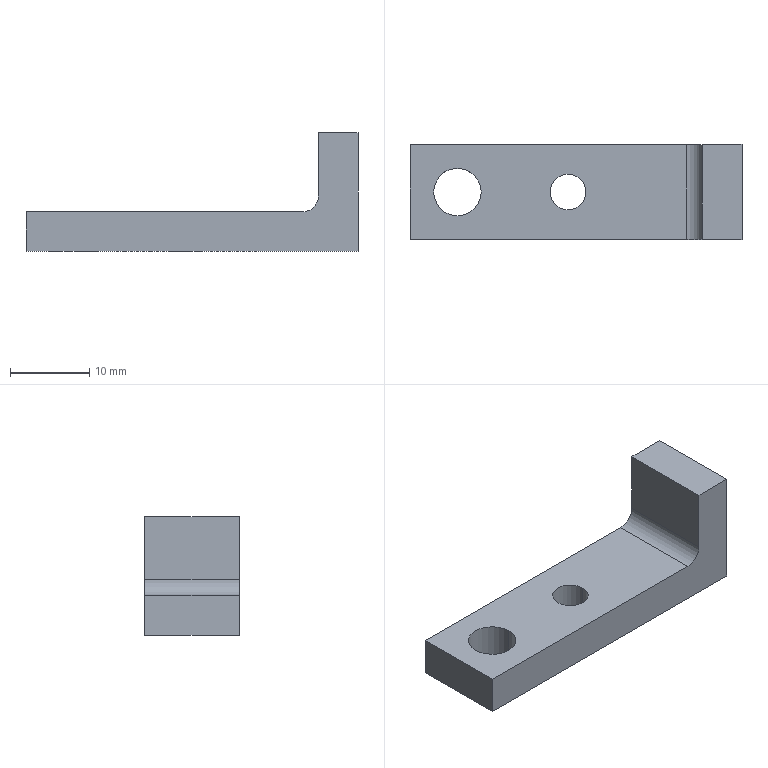Part | SolidWorks | features Extrusion 1, Fillet 1, ICE 1 | 1 solid | 13 faces | box 42 x 12 x 15 mm | volume 2909 mm3 | plane 8 | cylinder 5 | commonest cylinder face diameters 4.5 x2 6 x2 4 x1
STEP:
#1=CARTESIAN_POINT('',(3.,6.,5.));
#2=VERTEX_POINT('',#1);
#3=CARTESIAN_POINT('',(9.,6.,5.));
#4=VERTEX_POINT('',#3);
#5=CARTESIAN_POINT('',(6.,6.,5.));
#6=DIRECTION('',(0.,0.,1.));
#7=DIRECTION('',(1.,0.,0.));
#8=AXIS2_PLACEMENT_3D('',#5,#6,#7);
#9=CIRCLE('',#8,3.);
#10=EDGE_CURVE('',#2,#4,#9,.T.);
#11=ORIENTED_EDGE('',*,*,#10,.T.);
#12=CARTESIAN_POINT('',(9.,6.,0.));
#13=VERTEX_POINT('',#12);
#14=CARTESIAN_POINT('',(9.,6.,5.));
#15=DIRECTION('',(0.,0.,-1.));
#16=VECTOR('',#15,1000.);
#17=LINE('',#14,#16);
#18=EDGE_CURVE('',#4,#13,#17,.T.);
#19=ORIENTED_EDGE('',*,*,#18,.T.);
#20=CARTESIAN_POINT('',(3.,6.,0.));
#21=VERTEX_POINT('',#20);
#22=CARTESIAN_POINT('',(6.,6.,0.));
#23=DIRECTION('',(0.,0.,1.));
#24=DIRECTION('',(1.,0.,0.));
#25=AXIS2_PLACEMENT_3D('',#22,#23,#24);
#26=CIRCLE('',#25,3.);
#27=EDGE_CURVE('',#21,#13,#26,.T.);
#28=ORIENTED_EDGE('',*,*,#27,.F.);
#29=CARTESIAN_POINT('',(3.,6.,5.));
#30=DIRECTION('',(0.,0.,-1.));
#31=VECTOR('',#30,1000.);
#32=LINE('',#29,#31);
#33=EDGE_CURVE('',#2,#21,#32,.T.);
#34=ORIENTED_EDGE('',*,*,#33,.F.);
#35=EDGE_LOOP('',(#11,#19,#28,#34));
#36=FACE_OUTER_BOUND('',#35,.T.);
#37=CARTESIAN_POINT('',(6.,6.,5.));
#38=DIRECTION('',(0.,0.,-1.));
#39=DIRECTION('',(-1.,0.,0.));
#40=AXIS2_PLACEMENT_3D('',#37,#38,#39);
#41=CYLINDRICAL_SURFACE('',#40,3.);
#42=ADVANCED_FACE('',(#36),#41,.F.);
#43=CARTESIAN_POINT('',(17.75,6.,5.));
#44=VERTEX_POINT('',#43);
#45=CARTESIAN_POINT('',(22.25,6.,5.));
#46=VERTEX_POINT('',#45);
#47=CARTESIAN_POINT('',(20.,6.,5.));
#48=DIRECTION('',(0.,0.,1.));
#49=DIRECTION('',(1.,0.,0.));
#50=AXIS2_PLACEMENT_3D('',#47,#48,#49);
#51=CIRCLE('',#50,2.25);
#52=EDGE_CURVE('',#44,#46,#51,.T.);
#53=ORIENTED_EDGE('',*,*,#52,.T.);
#54=CARTESIAN_POINT('',(22.25,6.,0.));
#55=VERTEX_POINT('',#54);
#56=CARTESIAN_POINT('',(22.25,6.,5.));
#57=DIRECTION('',(0.,0.,-1.));
#58=VECTOR('',#57,1000.);
#59=LINE('',#56,#58);
#60=EDGE_CURVE('',#46,#55,#59,.T.);
#61=ORIENTED_EDGE('',*,*,#60,.T.);
#62=CARTESIAN_POINT('',(17.75,6.,0.));
#63=VERTEX_POINT('',#62);
#64=CARTESIAN_POINT('',(20.,6.,0.));
#65=DIRECTION('',(0.,0.,1.));
#66=DIRECTION('',(1.,0.,0.));
#67=AXIS2_PLACEMENT_3D('',#64,#65,#66);
#68=CIRCLE('',#67,2.25);
#69=EDGE_CURVE('',#63,#55,#68,.T.);
#70=ORIENTED_EDGE('',*,*,#69,.F.);
#71=CARTESIAN_POINT('',(17.75,6.,5.));
#72=DIRECTION('',(0.,0.,-1.));
#73=VECTOR('',#72,1000.);
#74=LINE('',#71,#73);
#75=EDGE_CURVE('',#44,#63,#74,.T.);
#76=ORIENTED_EDGE('',*,*,#75,.F.);
#77=EDGE_LOOP('',(#53,#61,#70,#76));
#78=FACE_OUTER_BOUND('',#77,.T.);
#79=CARTESIAN_POINT('',(20.,6.,5.));
#80=DIRECTION('',(0.,0.,-1.));
#81=DIRECTION('',(-1.,0.,0.));
#82=AXIS2_PLACEMENT_3D('',#79,#80,#81);
#83=CYLINDRICAL_SURFACE('',#82,2.25);
#84=ADVANCED_FACE('',(#78),#83,.F.);
#85=ORIENTED_EDGE('',*,*,#10,.F.);
#86=CARTESIAN_POINT('',(6.,6.,5.));
#87=DIRECTION('',(0.,0.,1.));
#88=DIRECTION('',(1.,0.,0.));
#89=AXIS2_PLACEMENT_3D('',#86,#87,#88);
#90=CIRCLE('',#89,3.);
#91=EDGE_CURVE('',#4,#2,#90,.T.);
#92=ORIENTED_EDGE('',*,*,#91,.F.);
#93=EDGE_LOOP('',(#85,#92));
#94=FACE_BOUND('',#93,.T.);
#95=ORIENTED_EDGE('',*,*,#52,.F.);
#96=CARTESIAN_POINT('',(20.,6.,5.));
#97=DIRECTION('',(0.,0.,1.));
#98=DIRECTION('',(1.,0.,0.));
#99=AXIS2_PLACEMENT_3D('',#96,#97,#98);
#100=CIRCLE('',#99,2.25);
#101=EDGE_CURVE('',#46,#44,#100,.T.);
#102=ORIENTED_EDGE('',*,*,#101,.F.);
#103=EDGE_LOOP('',(#95,#102));
#104=FACE_BOUND('',#103,.T.);
#105=CARTESIAN_POINT('',(0.,0.,5.));
#106=VERTEX_POINT('',#105);
#107=CARTESIAN_POINT('',(35.,0.,5.));
#108=VERTEX_POINT('',#107);
#109=CARTESIAN_POINT('',(0.,0.,5.));
#110=DIRECTION('',(1.,0.,0.));
#111=VECTOR('',#110,1000.);
#112=LINE('',#109,#111);
#113=EDGE_CURVE('',#106,#108,#112,.T.);
#114=ORIENTED_EDGE('',*,*,#113,.T.);
#115=CARTESIAN_POINT('',(35.,12.,5.));
#116=VERTEX_POINT('',#115);
#117=CARTESIAN_POINT('',(35.,12.,5.));
#118=DIRECTION('',(0.,1.,0.));
#119=VECTOR('',#118,1000.);
#120=LINE('',#117,#119);
#121=EDGE_CURVE('',#108,#116,#120,.T.);
#122=ORIENTED_EDGE('',*,*,#121,.T.);
#123=CARTESIAN_POINT('',(0.,12.,5.));
#124=VERTEX_POINT('',#123);
#125=CARTESIAN_POINT('',(0.,12.,5.));
#126=DIRECTION('',(-1.,0.,0.));
#127=VECTOR('',#126,1000.);
#128=LINE('',#125,#127);
#129=EDGE_CURVE('',#116,#124,#128,.T.);
#130=ORIENTED_EDGE('',*,*,#129,.T.);
#131=CARTESIAN_POINT('',(0.,0.,5.));
#132=DIRECTION('',(0.,-1.,0.));
#133=VECTOR('',#132,1000.);
#134=LINE('',#131,#133);
#135=EDGE_CURVE('',#124,#106,#134,.T.);
#136=ORIENTED_EDGE('',*,*,#135,.T.);
#137=EDGE_LOOP('',(#114,#122,#130,#136));
#138=FACE_OUTER_BOUND('',#137,.T.);
#139=CARTESIAN_POINT('',(0.,0.,5.));
#140=DIRECTION('',(0.,0.,-1.));
#141=DIRECTION('',(-1.,0.,0.));
#142=AXIS2_PLACEMENT_3D('',#139,#140,#141);
#143=PLANE('',#142);
#144=ADVANCED_FACE('',(#94,#104,#138),#143,.F.);
#145=ORIENTED_EDGE('',*,*,#69,.T.);
#146=CARTESIAN_POINT('',(20.,6.,0.));
#147=DIRECTION('',(0.,0.,1.));
#148=DIRECTION('',(1.,0.,0.));
#149=AXIS2_PLACEMENT_3D('',#146,#147,#148);
#150=CIRCLE('',#149,2.25);
#151=EDGE_CURVE('',#55,#63,#150,.T.);
#152=ORIENTED_EDGE('',*,*,#151,.T.);
#153=EDGE_LOOP('',(#145,#152));
#154=FACE_BOUND('',#153,.T.);
#155=CARTESIAN_POINT('',(0.,12.,0.));
#156=VERTEX_POINT('',#155);
#157=CARTESIAN_POINT('',(0.,0.,0.));
#158=VERTEX_POINT('',#157);
#159=CARTESIAN_POINT('',(0.,0.,0.));
#160=DIRECTION('',(0.,-1.,0.));
#161=VECTOR('',#160,1000.);
#162=LINE('',#159,#161);
#163=EDGE_CURVE('',#156,#158,#162,.T.);
#164=ORIENTED_EDGE('',*,*,#163,.F.);
#165=CARTESIAN_POINT('',(42.,12.,0.));
#166=VERTEX_POINT('',#165);
#167=CARTESIAN_POINT('',(0.,12.,0.));
#168=DIRECTION('',(-1.,0.,0.));
#169=VECTOR('',#168,1000.);
#170=LINE('',#167,#169);
#171=EDGE_CURVE('',#166,#156,#170,.T.);
#172=ORIENTED_EDGE('',*,*,#171,.F.);
#173=CARTESIAN_POINT('',(42.,0.,0.));
#174=VERTEX_POINT('',#173);
#175=CARTESIAN_POINT('',(42.,0.,0.));
#176=DIRECTION('',(0.,1.,0.));
#177=VECTOR('',#176,1000.);
#178=LINE('',#175,#177);
#179=EDGE_CURVE('',#174,#166,#178,.T.);
#180=ORIENTED_EDGE('',*,*,#179,.F.);
#181=CARTESIAN_POINT('',(0.,0.,0.));
#182=DIRECTION('',(1.,0.,0.));
#183=VECTOR('',#182,1000.);
#184=LINE('',#181,#183);
#185=EDGE_CURVE('',#158,#174,#184,.T.);
#186=ORIENTED_EDGE('',*,*,#185,.F.);
#187=EDGE_LOOP('',(#164,#172,#180,#186));
#188=FACE_OUTER_BOUND('',#187,.T.);
#189=ORIENTED_EDGE('',*,*,#27,.T.);
#190=CARTESIAN_POINT('',(6.,6.,0.));
#191=DIRECTION('',(0.,0.,1.));
#192=DIRECTION('',(1.,0.,0.));
#193=AXIS2_PLACEMENT_3D('',#190,#191,#192);
#194=CIRCLE('',#193,3.);
#195=EDGE_CURVE('',#13,#21,#194,.T.);
#196=ORIENTED_EDGE('',*,*,#195,.T.);
#197=EDGE_LOOP('',(#189,#196));
#198=FACE_BOUND('',#197,.T.);
#199=CARTESIAN_POINT('',(0.,0.,0.));
#200=DIRECTION('',(0.,0.,-1.));
#201=DIRECTION('',(-1.,0.,0.));
#202=AXIS2_PLACEMENT_3D('',#199,#200,#201);
#203=PLANE('',#202);
#204=ADVANCED_FACE('',(#154,#188,#198),#203,.T.);
#205=ORIENTED_EDGE('',*,*,#163,.T.);
#206=CARTESIAN_POINT('',(0.,0.,5.));
#207=DIRECTION('',(0.,0.,-1.));
#208=VECTOR('',#207,1000.);
#209=LINE('',#206,#208);
#210=EDGE_CURVE('',#106,#158,#209,.T.);
#211=ORIENTED_EDGE('',*,*,#210,.F.);
#212=ORIENTED_EDGE('',*,*,#135,.F.);
#213=CARTESIAN_POINT('',(0.,12.,5.));
#214=DIRECTION('',(0.,0.,-1.));
#215=VECTOR('',#214,1000.);
#216=LINE('',#213,#215);
#217=EDGE_CURVE('',#124,#156,#216,.T.);
#218=ORIENTED_EDGE('',*,*,#217,.T.);
#219=EDGE_LOOP('',(#205,#211,#212,#218));
#220=FACE_OUTER_BOUND('',#219,.T.);
#221=CARTESIAN_POINT('',(0.,0.,5.));
#222=DIRECTION('',(1.,0.,0.));
#223=DIRECTION('',(0.,0.,-1.));
#224=AXIS2_PLACEMENT_3D('',#221,#222,#223);
#225=PLANE('',#224);
#226=ADVANCED_FACE('',(#220),#225,.F.);
#227=ORIENTED_EDGE('',*,*,#185,.T.);
#228=CARTESIAN_POINT('',(42.,0.,15.));
#229=VERTEX_POINT('',#228);
#230=CARTESIAN_POINT('',(42.,0.,5.));
#231=DIRECTION('',(0.,0.,-1.));
#232=VECTOR('',#231,1000.);
#233=LINE('',#230,#232);
#234=EDGE_CURVE('',#229,#174,#233,.T.);
#235=ORIENTED_EDGE('',*,*,#234,.F.);
#236=CARTESIAN_POINT('',(37.,0.,15.));
#237=VERTEX_POINT('',#236);
#238=CARTESIAN_POINT('',(42.,0.,15.));
#239=DIRECTION('',(1.,0.,0.));
#240=VECTOR('',#239,1000.);
#241=LINE('',#238,#240);
#242=EDGE_CURVE('',#237,#229,#241,.T.);
#243=ORIENTED_EDGE('',*,*,#242,.F.);
#244=CARTESIAN_POINT('',(37.,0.,7.));
#245=VERTEX_POINT('',#244);
#246=CARTESIAN_POINT('',(37.,0.,15.));
#247=DIRECTION('',(0.,0.,-1.));
#248=VECTOR('',#247,1000.);
#249=LINE('',#246,#248);
#250=EDGE_CURVE('',#237,#245,#249,.T.);
#251=ORIENTED_EDGE('',*,*,#250,.T.);
#252=CARTESIAN_POINT('',(35.,0.,7.));
#253=DIRECTION('',(0.,1.,0.));
#254=DIRECTION('',(0.,0.,1.));
#255=AXIS2_PLACEMENT_3D('',#252,#253,#254);
#256=CIRCLE('',#255,2.);
#257=EDGE_CURVE('',#245,#108,#256,.T.);
#258=ORIENTED_EDGE('',*,*,#257,.T.);
#259=ORIENTED_EDGE('',*,*,#113,.F.);
#260=ORIENTED_EDGE('',*,*,#210,.T.);
#261=EDGE_LOOP('',(#227,#235,#243,#251,#258,#259,#260));
#262=FACE_OUTER_BOUND('',#261,.T.);
#263=CARTESIAN_POINT('',(0.,0.,5.));
#264=DIRECTION('',(0.,1.,0.));
#265=DIRECTION('',(0.,0.,1.));
#266=AXIS2_PLACEMENT_3D('',#263,#264,#265);
#267=PLANE('',#266);
#268=ADVANCED_FACE('',(#262),#267,.F.);
#269=ORIENTED_EDGE('',*,*,#179,.T.);
#270=CARTESIAN_POINT('',(42.,12.,15.));
#271=VERTEX_POINT('',#270);
#272=CARTESIAN_POINT('',(42.,12.,5.));
#273=DIRECTION('',(0.,0.,-1.));
#274=VECTOR('',#273,1000.);
#275=LINE('',#272,#274);
#276=EDGE_CURVE('',#271,#166,#275,.T.);
#277=ORIENTED_EDGE('',*,*,#276,.F.);
#278=CARTESIAN_POINT('',(42.,0.,15.));
#279=DIRECTION('',(0.,1.,0.));
#280=VECTOR('',#279,1000.);
#281=LINE('',#278,#280);
#282=EDGE_CURVE('',#229,#271,#281,.T.);
#283=ORIENTED_EDGE('',*,*,#282,.F.);
#284=ORIENTED_EDGE('',*,*,#234,.T.);
#285=EDGE_LOOP('',(#269,#277,#283,#284));
#286=FACE_OUTER_BOUND('',#285,.T.);
#287=CARTESIAN_POINT('',(42.,0.,5.));
#288=DIRECTION('',(-1.,0.,0.));
#289=DIRECTION('',(0.,0.,1.));
#290=AXIS2_PLACEMENT_3D('',#287,#288,#289);
#291=PLANE('',#290);
#292=ADVANCED_FACE('',(#286),#291,.F.);
#293=ORIENTED_EDGE('',*,*,#171,.T.);
#294=ORIENTED_EDGE('',*,*,#217,.F.);
#295=ORIENTED_EDGE('',*,*,#129,.F.);
#296=CARTESIAN_POINT('',(37.,12.,7.));
#297=VERTEX_POINT('',#296);
#298=CARTESIAN_POINT('',(35.,12.,7.));
#299=DIRECTION('',(0.,-1.,0.));
#300=DIRECTION('',(0.,0.,-1.));
#301=AXIS2_PLACEMENT_3D('',#298,#299,#300);
#302=CIRCLE('',#301,2.);
#303=EDGE_CURVE('',#116,#297,#302,.T.);
#304=ORIENTED_EDGE('',*,*,#303,.T.);
#305=CARTESIAN_POINT('',(37.,12.,15.));
#306=VERTEX_POINT('',#305);
#307=CARTESIAN_POINT('',(37.,12.,15.));
#308=DIRECTION('',(0.,0.,-1.));
#309=VECTOR('',#308,1000.);
#310=LINE('',#307,#309);
#311=EDGE_CURVE('',#306,#297,#310,.T.);
#312=ORIENTED_EDGE('',*,*,#311,.F.);
#313=CARTESIAN_POINT('',(42.,12.,15.));
#314=DIRECTION('',(-1.,0.,0.));
#315=VECTOR('',#314,1000.);
#316=LINE('',#313,#315);
#317=EDGE_CURVE('',#271,#306,#316,.T.);
#318=ORIENTED_EDGE('',*,*,#317,.F.);
#319=ORIENTED_EDGE('',*,*,#276,.T.);
#320=EDGE_LOOP('',(#293,#294,#295,#304,#312,#318,#319));
#321=FACE_OUTER_BOUND('',#320,.T.);
#322=CARTESIAN_POINT('',(0.,12.,5.));
#323=DIRECTION('',(0.,-1.,0.));
#324=DIRECTION('',(0.,0.,-1.));
#325=AXIS2_PLACEMENT_3D('',#322,#323,#324);
#326=PLANE('',#325);
#327=ADVANCED_FACE('',(#321),#326,.F.);
#328=ORIENTED_EDGE('',*,*,#60,.F.);
#329=ORIENTED_EDGE('',*,*,#101,.T.);
#330=ORIENTED_EDGE('',*,*,#75,.T.);
#331=ORIENTED_EDGE('',*,*,#151,.F.);
#332=EDGE_LOOP('',(#328,#329,#330,#331));
#333=FACE_OUTER_BOUND('',#332,.T.);
#334=CARTESIAN_POINT('',(20.,6.,5.));
#335=DIRECTION('',(0.,0.,-1.));
#336=DIRECTION('',(-1.,0.,0.));
#337=AXIS2_PLACEMENT_3D('',#334,#335,#336);
#338=CYLINDRICAL_SURFACE('',#337,2.25);
#339=ADVANCED_FACE('',(#333),#338,.F.);
#340=ORIENTED_EDGE('',*,*,#18,.F.);
#341=ORIENTED_EDGE('',*,*,#91,.T.);
#342=ORIENTED_EDGE('',*,*,#33,.T.);
#343=ORIENTED_EDGE('',*,*,#195,.F.);
#344=EDGE_LOOP('',(#340,#341,#342,#343));
#345=FACE_OUTER_BOUND('',#344,.T.);
#346=CARTESIAN_POINT('',(6.,6.,5.));
#347=DIRECTION('',(0.,0.,-1.));
#348=DIRECTION('',(-1.,0.,0.));
#349=AXIS2_PLACEMENT_3D('',#346,#347,#348);
#350=CYLINDRICAL_SURFACE('',#349,3.);
#351=ADVANCED_FACE('',(#345),#350,.F.);
#352=ORIENTED_EDGE('',*,*,#311,.T.);
#353=CARTESIAN_POINT('',(37.,0.,7.));
#354=DIRECTION('',(0.,-1.,0.));
#355=VECTOR('',#354,1000.);
#356=LINE('',#353,#355);
#357=EDGE_CURVE('',#297,#245,#356,.T.);
#358=ORIENTED_EDGE('',*,*,#357,.T.);
#359=ORIENTED_EDGE('',*,*,#250,.F.);
#360=CARTESIAN_POINT('',(37.,0.,15.));
#361=DIRECTION('',(0.,-1.,0.));
#362=VECTOR('',#361,1000.);
#363=LINE('',#360,#362);
#364=EDGE_CURVE('',#306,#237,#363,.T.);
#365=ORIENTED_EDGE('',*,*,#364,.F.);
#366=EDGE_LOOP('',(#352,#358,#359,#365));
#367=FACE_OUTER_BOUND('',#366,.T.);
#368=CARTESIAN_POINT('',(37.,0.,15.));
#369=DIRECTION('',(1.,0.,0.));
#370=DIRECTION('',(0.,0.,-1.));
#371=AXIS2_PLACEMENT_3D('',#368,#369,#370);
#372=PLANE('',#371);
#373=ADVANCED_FACE('',(#367),#372,.F.);
#374=ORIENTED_EDGE('',*,*,#282,.T.);
#375=ORIENTED_EDGE('',*,*,#317,.T.);
#376=ORIENTED_EDGE('',*,*,#364,.T.);
#377=ORIENTED_EDGE('',*,*,#242,.T.);
#378=EDGE_LOOP('',(#374,#375,#376,#377));
#379=FACE_OUTER_BOUND('',#378,.T.);
#380=CARTESIAN_POINT('',(0.,0.,15.));
#381=DIRECTION('',(0.,0.,1.));
#382=DIRECTION('',(1.,0.,0.));
#383=AXIS2_PLACEMENT_3D('',#380,#381,#382);
#384=PLANE('',#383);
#385=ADVANCED_FACE('',(#379),#384,.T.);
#386=ORIENTED_EDGE('',*,*,#303,.F.);
#387=ORIENTED_EDGE('',*,*,#121,.F.);
#388=ORIENTED_EDGE('',*,*,#257,.F.);
#389=ORIENTED_EDGE('',*,*,#357,.F.);
#390=EDGE_LOOP('',(#386,#387,#388,#389));
#391=FACE_OUTER_BOUND('',#390,.T.);
#392=CARTESIAN_POINT('',(35.,0.,7.));
#393=DIRECTION('',(0.,1.,0.));
#394=DIRECTION('',(0.,0.,1.));
#395=AXIS2_PLACEMENT_3D('',#392,#393,#394);
#396=CYLINDRICAL_SURFACE('',#395,2.);
#397=ADVANCED_FACE('',(#391),#396,.F.);
#398=CLOSED_SHELL('',(#42,#84,#144,#204,#226,#268,#292,#327,#339,#351,#373,#385,#397));
#399=MANIFOLD_SOLID_BREP('',#398);
#400=CARTESIAN_POINT('',(0.,0.,0.));
#401=DIRECTION('',(0.,0.,1.));
#402=DIRECTION('',(1.,0.,0.));
#403=AXIS2_PLACEMENT_3D('',#400,#401,#402);
#404=(LENGTH_UNIT()NAMED_UNIT(*)SI_UNIT(.MILLI.,.METRE.));
#405=UNCERTAINTY_MEASURE_WITH_UNIT(LENGTH_MEASURE(0.00001),#404,'','');
#406=(NAMED_UNIT(*)PLANE_ANGLE_UNIT()SI_UNIT($,.RADIAN.));
#407=(NAMED_UNIT(*)SI_UNIT($,.STERADIAN.)SOLID_ANGLE_UNIT());
#408=(GEOMETRIC_REPRESENTATION_CONTEXT(3)GLOBAL_UNCERTAINTY_ASSIGNED_CONTEXT((#405))GLOBAL_UNIT_ASSIGNED_CONTEXT((#404,#406,#407))REPRESENTATION_CONTEXT('',''));
#409=ADVANCED_BREP_SHAPE_REPRESENTATION('',(#399,#403),#408);